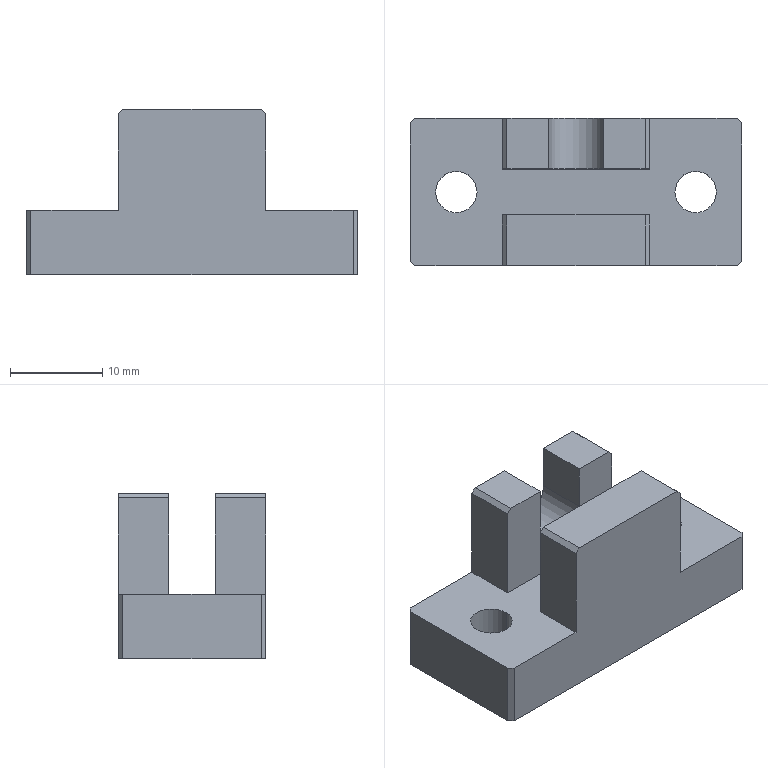Part | STEP file | PN_0009 Mount electronic clip movable connector head B | 1 solid | 30 faces | box 36 x 16 x 18 mm | volume 5496 mm3 | plane 25 | cylinder 5 | commonest cylinder face diameters 4.5 x4 6 x1